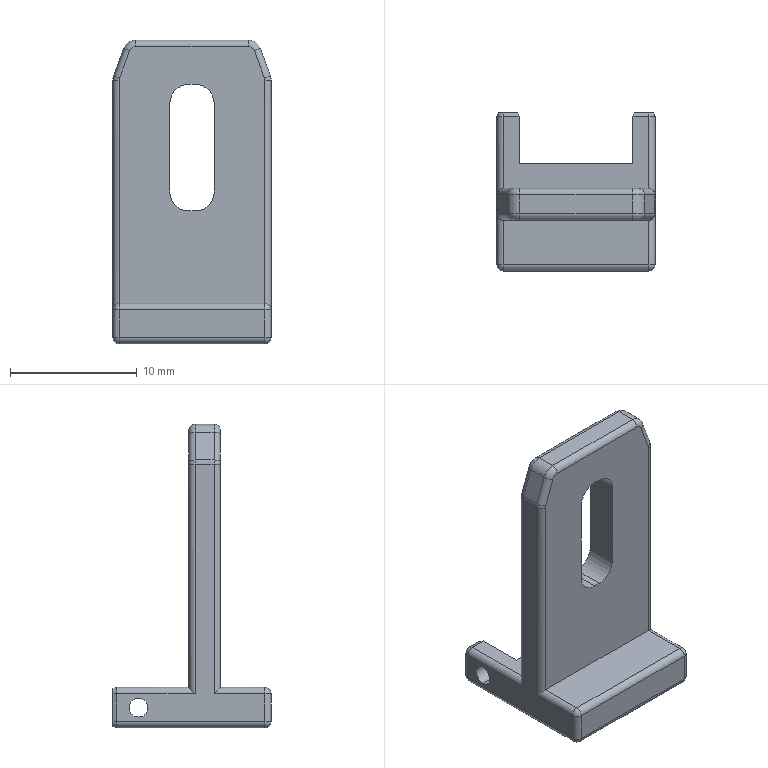Part | SolidWorks | features ICE 4, Fillet 3, Chamfer 2, Cut 1, Extrusion 1 | 1 solid | 76 faces | box 12.5 x 12.5 x 24 mm | volume 927.398 mm3 | cylinder 32 | plane 28 | torus 8 | sphere 4 | cone 4 | commonest cylinder face diameters 1 x20 1.5 x4 2 x4 3 x4